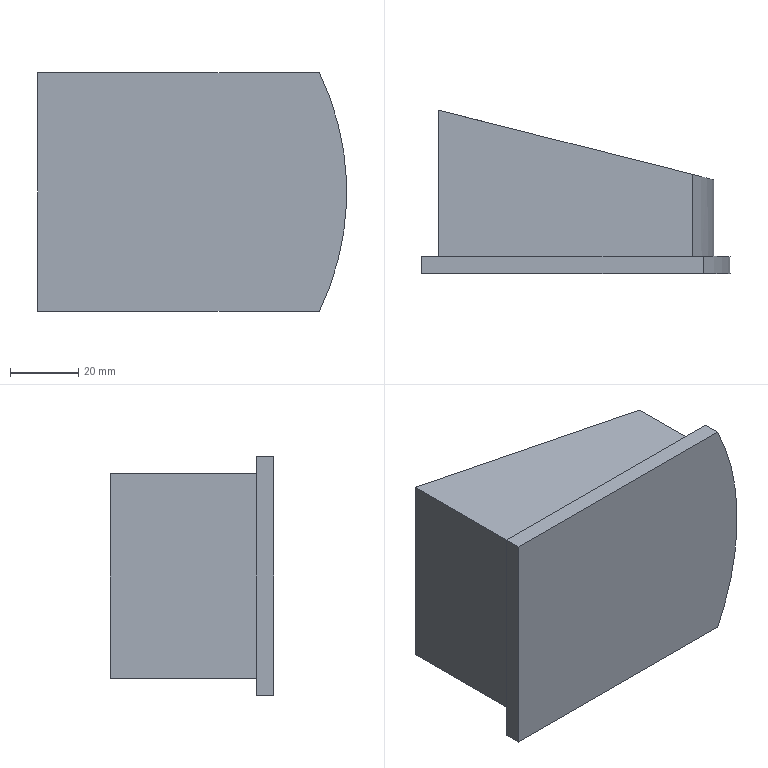Part | SolidWorks | features ICE 4, Extrusion 1, Fillet 1 | 1 solid | 43 faces | box 90.603 x 47.87 x 70 mm | volume 179033 mm3 | cylinder 18 | plane 17 | spline 8 | commonest cylinder face diameters 6 x8 10 x8 150 x1 160 x1